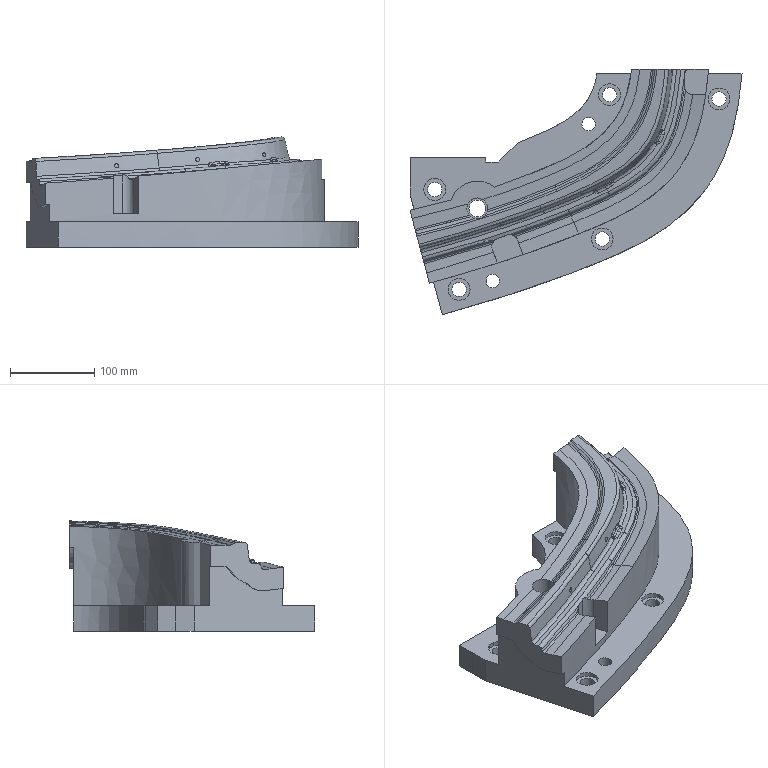Part | NX | features solid 2 | 1 solid | 139 faces | box 394.547 x 291.367 x 130.951 mm | volume 4476825 mm3 | spline 91 | plane 28 | cylinder 20 | commonest cylinder face diameters 17 x5 20 x5 26 x5 16 x2 25 x1 28 x1